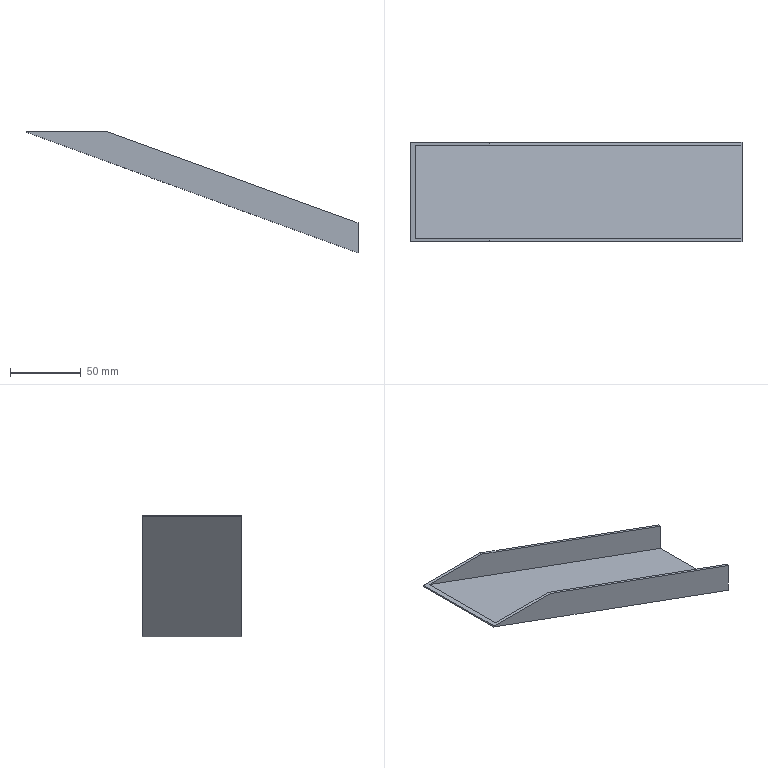Part | NX | features solid 2 | 1 solid | 11 faces | box 233.969 x 70 x 85.956 mm | volume 50310 mm3 | plane 11
STEP:
#1=CARTESIAN_POINT('',(406.321,-180.,-155.));
#2=VERTEX_POINT('',#1);
#3=CARTESIAN_POINT('',(406.031,-180.,-155.798));
#4=VERTEX_POINT('',#3);
#5=CARTESIAN_POINT('',(406.715,-180.,-153.919));
#6=DIRECTION('',(-0.342,0.,-0.9397));
#7=VECTOR('',#6,1000.);
#8=LINE('',#5,#7);
#9=EDGE_CURVE('',#2,#4,#8,.T.);
#10=ORIENTED_EDGE('',*,*,#9,.T.);
#11=CARTESIAN_POINT('',(640.,-180.,-240.956));
#12=VERTEX_POINT('',#11);
#13=CARTESIAN_POINT('',(1313.3,-180.,-486.017));
#14=DIRECTION('',(-0.9397,0.,0.342));
#15=VECTOR('',#14,1000.);
#16=LINE('',#13,#15);
#17=EDGE_CURVE('',#12,#4,#16,.T.);
#18=ORIENTED_EDGE('',*,*,#17,.F.);
#19=CARTESIAN_POINT('',(640.,-180.,-219.672));
#20=VERTEX_POINT('',#19);
#21=CARTESIAN_POINT('',(640.,-180.,-226.397));
#22=DIRECTION('',(0.,0.,1.));
#23=VECTOR('',#22,1000.);
#24=LINE('',#21,#23);
#25=EDGE_CURVE('',#12,#20,#24,.T.);
#26=ORIENTED_EDGE('',*,*,#25,.T.);
#27=CARTESIAN_POINT('',(462.314,-180.,-155.));
#28=VERTEX_POINT('',#27);
#29=CARTESIAN_POINT('',(2083.44,-180.,-745.042));
#30=DIRECTION('',(-0.9397,0.,0.342));
#31=VECTOR('',#30,1000.);
#32=LINE('',#29,#31);
#33=EDGE_CURVE('',#20,#28,#32,.T.);
#34=ORIENTED_EDGE('',*,*,#33,.T.);
#35=CARTESIAN_POINT('',(2077.284,-180.,-155.));
#36=DIRECTION('',(-1.,0.,0.));
#37=VECTOR('',#36,1000.);
#38=LINE('',#35,#37);
#39=EDGE_CURVE('',#2,#28,#38,.F.);
#40=ORIENTED_EDGE('',*,*,#39,.F.);
#41=EDGE_LOOP('',(#10,#18,#26,#34,#40));
#42=FACE_BOUND('',#41,.T.);
#43=CARTESIAN_POINT('',(2077.284,-180.,-761.956));
#44=DIRECTION('',(0.,1.,0.));
#45=DIRECTION('',(0.,0.,1.));
#46=AXIS2_PLACEMENT_3D('',#43,#44,#45);
#47=PLANE('',#46);
#48=ADVANCED_FACE('',(#42),#47,.F.);
#49=CARTESIAN_POINT('',(406.321,-110.,-155.));
#50=VERTEX_POINT('',#49);
#51=CARTESIAN_POINT('',(462.314,-110.,-155.));
#52=VERTEX_POINT('',#51);
#53=CARTESIAN_POINT('',(2077.284,-110.,-155.));
#54=DIRECTION('',(-1.,0.,0.));
#55=VECTOR('',#54,1000.);
#56=LINE('',#53,#55);
#57=EDGE_CURVE('',#50,#52,#56,.F.);
#58=ORIENTED_EDGE('',*,*,#57,.T.);
#59=CARTESIAN_POINT('',(640.,-110.,-219.672));
#60=VERTEX_POINT('',#59);
#61=CARTESIAN_POINT('',(606.84,-110.,-207.603));
#62=DIRECTION('',(-0.9397,0.,0.342));
#63=VECTOR('',#62,1000.);
#64=LINE('',#61,#63);
#65=EDGE_CURVE('',#60,#52,#64,.T.);
#66=ORIENTED_EDGE('',*,*,#65,.F.);
#67=CARTESIAN_POINT('',(640.,-110.,-240.956));
#68=VERTEX_POINT('',#67);
#69=CARTESIAN_POINT('',(640.,-110.,-226.397));
#70=DIRECTION('',(0.,0.,1.));
#71=VECTOR('',#70,1000.);
#72=LINE('',#69,#71);
#73=EDGE_CURVE('',#68,#60,#72,.T.);
#74=ORIENTED_EDGE('',*,*,#73,.F.);
#75=CARTESIAN_POINT('',(406.031,-110.,-155.798));
#76=VERTEX_POINT('',#75);
#77=CARTESIAN_POINT('',(1313.3,-110.,-486.017));
#78=DIRECTION('',(-0.9397,0.,0.342));
#79=VECTOR('',#78,1000.);
#80=LINE('',#77,#79);
#81=EDGE_CURVE('',#68,#76,#80,.T.);
#82=ORIENTED_EDGE('',*,*,#81,.T.);
#83=CARTESIAN_POINT('',(406.715,-110.,-153.919));
#84=DIRECTION('',(-0.342,0.,-0.9397));
#85=VECTOR('',#84,1000.);
#86=LINE('',#83,#85);
#87=EDGE_CURVE('',#50,#76,#86,.T.);
#88=ORIENTED_EDGE('',*,*,#87,.F.);
#89=EDGE_LOOP('',(#58,#66,#74,#82,#88));
#90=FACE_BOUND('',#89,.T.);
#91=CARTESIAN_POINT('',(2077.284,-110.,-761.956));
#92=DIRECTION('',(0.,1.,0.));
#93=DIRECTION('',(0.,0.,1.));
#94=AXIS2_PLACEMENT_3D('',#91,#92,#93);
#95=PLANE('',#94);
#96=ADVANCED_FACE('',(#90),#95,.T.);
#97=ORIENTED_EDGE('',*,*,#87,.T.);
#98=CARTESIAN_POINT('',(406.031,-706.946,-155.798));
#99=DIRECTION('',(0.,1.,0.));
#100=VECTOR('',#99,1000.);
#101=LINE('',#98,#100);
#102=EDGE_CURVE('',#4,#76,#101,.T.);
#103=ORIENTED_EDGE('',*,*,#102,.F.);
#104=ORIENTED_EDGE('',*,*,#9,.F.);
#105=CARTESIAN_POINT('',(406.321,-2357.783,-155.));
#106=DIRECTION('',(0.,1.,0.));
#107=VECTOR('',#106,1000.);
#108=LINE('',#105,#107);
#109=EDGE_CURVE('',#50,#2,#108,.F.);
#110=ORIENTED_EDGE('',*,*,#109,.F.);
#111=EDGE_LOOP('',(#97,#103,#104,#110));
#112=FACE_BOUND('',#111,.T.);
#113=CARTESIAN_POINT('',(406.715,-2357.783,-153.919));
#114=DIRECTION('',(0.9397,0.,-0.342));
#115=DIRECTION('',(0.342,0.,0.9397));
#116=AXIS2_PLACEMENT_3D('',#113,#114,#115);
#117=PLANE('',#116);
#118=ADVANCED_FACE('',(#112),#117,.F.);
#119=CARTESIAN_POINT('',(640.,-112.,-238.827));
#120=VERTEX_POINT('',#119);
#121=CARTESIAN_POINT('',(409.686,-112.,-155.));
#122=VERTEX_POINT('',#121);
#123=CARTESIAN_POINT('',(1313.984,-112.,-484.138));
#124=DIRECTION('',(-0.9397,0.,0.342));
#125=VECTOR('',#124,1000.);
#126=LINE('',#123,#125);
#127=EDGE_CURVE('',#120,#122,#126,.T.);
#128=ORIENTED_EDGE('',*,*,#127,.F.);
#129=CARTESIAN_POINT('',(640.,-112.,-219.672));
#130=VERTEX_POINT('',#129);
#131=CARTESIAN_POINT('',(640.,-112.,-226.397));
#132=DIRECTION('',(0.,0.,-1.));
#133=VECTOR('',#132,1000.);
#134=LINE('',#131,#133);
#135=EDGE_CURVE('',#130,#120,#134,.T.);
#136=ORIENTED_EDGE('',*,*,#135,.F.);
#137=CARTESIAN_POINT('',(462.314,-112.,-155.));
#138=VERTEX_POINT('',#137);
#139=CARTESIAN_POINT('',(606.84,-112.,-207.603));
#140=DIRECTION('',(-0.9397,0.,0.342));
#141=VECTOR('',#140,1000.);
#142=LINE('',#139,#141);
#143=EDGE_CURVE('',#130,#138,#142,.T.);
#144=ORIENTED_EDGE('',*,*,#143,.T.);
#145=CARTESIAN_POINT('',(600.,-112.,-155.));
#146=DIRECTION('',(-1.,0.,0.));
#147=VECTOR('',#146,1000.);
#148=LINE('',#145,#147);
#149=EDGE_CURVE('',#122,#138,#148,.F.);
#150=ORIENTED_EDGE('',*,*,#149,.F.);
#151=EDGE_LOOP('',(#128,#136,#144,#150));
#152=FACE_BOUND('',#151,.T.);
#153=CARTESIAN_POINT('',(600.,-112.,-226.397));
#154=DIRECTION('',(0.,1.,0.));
#155=DIRECTION('',(-0.9397,0.,0.342));
#156=AXIS2_PLACEMENT_3D('',#153,#154,#155);
#157=PLANE('',#156);
#158=ADVANCED_FACE('',(#152),#157,.F.);
#159=ORIENTED_EDGE('',*,*,#143,.F.);
#160=CARTESIAN_POINT('',(640.,-90.,-219.672));
#161=DIRECTION('',(0.,-1.,0.));
#162=VECTOR('',#161,1000.);
#163=LINE('',#160,#162);
#164=EDGE_CURVE('',#60,#130,#163,.T.);
#165=ORIENTED_EDGE('',*,*,#164,.F.);
#166=ORIENTED_EDGE('',*,*,#65,.T.);
#167=CARTESIAN_POINT('',(462.314,-90.,-155.));
#168=DIRECTION('',(0.,-1.,0.));
#169=VECTOR('',#168,1000.);
#170=LINE('',#167,#169);
#171=EDGE_CURVE('',#138,#52,#170,.F.);
#172=ORIENTED_EDGE('',*,*,#171,.F.);
#173=EDGE_LOOP('',(#159,#165,#166,#172));
#174=FACE_BOUND('',#173,.T.);
#175=CARTESIAN_POINT('',(606.84,-90.,-207.603));
#176=DIRECTION('',(-0.342,0.,-0.9397));
#177=DIRECTION('',(0.9397,0.,-0.342));
#178=AXIS2_PLACEMENT_3D('',#175,#176,#177);
#179=PLANE('',#178);
#180=ADVANCED_FACE('',(#174),#179,.F.);
#181=CARTESIAN_POINT('',(640.,-178.,-219.672));
#182=VERTEX_POINT('',#181);
#183=CARTESIAN_POINT('',(462.314,-178.,-155.));
#184=VERTEX_POINT('',#183);
#185=CARTESIAN_POINT('',(606.84,-178.,-207.603));
#186=DIRECTION('',(-0.9397,0.,0.342));
#187=VECTOR('',#186,1000.);
#188=LINE('',#185,#187);
#189=EDGE_CURVE('',#182,#184,#188,.T.);
#190=ORIENTED_EDGE('',*,*,#189,.F.);
#191=CARTESIAN_POINT('',(640.,-178.,-238.827));
#192=VERTEX_POINT('',#191);
#193=CARTESIAN_POINT('',(640.,-178.,-226.397));
#194=DIRECTION('',(0.,0.,1.));
#195=VECTOR('',#194,1000.);
#196=LINE('',#193,#195);
#197=EDGE_CURVE('',#192,#182,#196,.T.);
#198=ORIENTED_EDGE('',*,*,#197,.F.);
#199=CARTESIAN_POINT('',(409.686,-178.,-155.));
#200=VERTEX_POINT('',#199);
#201=CARTESIAN_POINT('',(1313.984,-178.,-484.138));
#202=DIRECTION('',(0.9397,0.,-0.342));
#203=VECTOR('',#202,1000.);
#204=LINE('',#201,#203);
#205=EDGE_CURVE('',#200,#192,#204,.T.);
#206=ORIENTED_EDGE('',*,*,#205,.F.);
#207=CARTESIAN_POINT('',(600.,-178.,-155.));
#208=DIRECTION('',(1.,0.,0.));
#209=VECTOR('',#208,1000.);
#210=LINE('',#207,#209);
#211=EDGE_CURVE('',#184,#200,#210,.F.);
#212=ORIENTED_EDGE('',*,*,#211,.F.);
#213=EDGE_LOOP('',(#190,#198,#206,#212));
#214=FACE_BOUND('',#213,.T.);
#215=CARTESIAN_POINT('',(600.,-178.,-226.397));
#216=DIRECTION('',(0.,-1.,0.));
#217=DIRECTION('',(-0.9397,0.,0.342));
#218=AXIS2_PLACEMENT_3D('',#215,#216,#217);
#219=PLANE('',#218);
#220=ADVANCED_FACE('',(#214),#219,.F.);
#221=CARTESIAN_POINT('',(462.314,-190.,-155.));
#222=DIRECTION('',(0.,1.,0.));
#223=VECTOR('',#222,1000.);
#224=LINE('',#221,#223);
#225=EDGE_CURVE('',#184,#28,#224,.F.);
#226=ORIENTED_EDGE('',*,*,#225,.T.);
#227=ORIENTED_EDGE('',*,*,#33,.F.);
#228=CARTESIAN_POINT('',(640.,-190.,-219.672));
#229=DIRECTION('',(0.,1.,0.));
#230=VECTOR('',#229,1000.);
#231=LINE('',#228,#230);
#232=EDGE_CURVE('',#20,#182,#231,.T.);
#233=ORIENTED_EDGE('',*,*,#232,.T.);
#234=ORIENTED_EDGE('',*,*,#189,.T.);
#235=EDGE_LOOP('',(#226,#227,#233,#234));
#236=FACE_BOUND('',#235,.T.);
#237=CARTESIAN_POINT('',(606.84,-190.,-207.603));
#238=DIRECTION('',(0.342,0.,0.9397));
#239=DIRECTION('',(-0.9397,0.,0.342));
#240=AXIS2_PLACEMENT_3D('',#237,#238,#239);
#241=PLANE('',#240);
#242=ADVANCED_FACE('',(#236),#241,.T.);
#243=ORIENTED_EDGE('',*,*,#205,.T.);
#244=CARTESIAN_POINT('',(640.,-706.946,-238.827));
#245=DIRECTION('',(0.,-1.,0.));
#246=VECTOR('',#245,1000.);
#247=LINE('',#244,#246);
#248=EDGE_CURVE('',#120,#192,#247,.T.);
#249=ORIENTED_EDGE('',*,*,#248,.F.);
#250=ORIENTED_EDGE('',*,*,#127,.T.);
#251=CARTESIAN_POINT('',(409.686,-706.946,-155.));
#252=DIRECTION('',(0.,-1.,0.));
#253=VECTOR('',#252,1000.);
#254=LINE('',#251,#253);
#255=EDGE_CURVE('',#200,#122,#254,.F.);
#256=ORIENTED_EDGE('',*,*,#255,.F.);
#257=EDGE_LOOP('',(#243,#249,#250,#256));
#258=FACE_BOUND('',#257,.T.);
#259=CARTESIAN_POINT('',(1313.984,-706.946,-484.138));
#260=DIRECTION('',(-0.342,0.,-0.9397));
#261=DIRECTION('',(0.9397,0.,-0.342));
#262=AXIS2_PLACEMENT_3D('',#259,#260,#261);
#263=PLANE('',#262);
#264=ADVANCED_FACE('',(#258),#263,.F.);
#265=CARTESIAN_POINT('',(640.,-190.,-240.956));
#266=DIRECTION('',(0.,1.,0.));
#267=VECTOR('',#266,1000.);
#268=LINE('',#265,#267);
#269=EDGE_CURVE('',#12,#68,#268,.T.);
#270=ORIENTED_EDGE('',*,*,#269,.F.);
#271=ORIENTED_EDGE('',*,*,#17,.T.);
#272=ORIENTED_EDGE('',*,*,#102,.T.);
#273=ORIENTED_EDGE('',*,*,#81,.F.);
#274=EDGE_LOOP('',(#270,#271,#272,#273));
#275=FACE_BOUND('',#274,.T.);
#276=CARTESIAN_POINT('',(1313.3,-706.946,-486.017));
#277=DIRECTION('',(-0.342,0.,-0.9397));
#278=DIRECTION('',(0.9397,0.,-0.342));
#279=AXIS2_PLACEMENT_3D('',#276,#277,#278);
#280=PLANE('',#279);
#281=ADVANCED_FACE('',(#275),#280,.T.);
#282=ORIENTED_EDGE('',*,*,#73,.T.);
#283=ORIENTED_EDGE('',*,*,#164,.T.);
#284=ORIENTED_EDGE('',*,*,#135,.T.);
#285=ORIENTED_EDGE('',*,*,#248,.T.);
#286=ORIENTED_EDGE('',*,*,#197,.T.);
#287=ORIENTED_EDGE('',*,*,#232,.F.);
#288=ORIENTED_EDGE('',*,*,#25,.F.);
#289=ORIENTED_EDGE('',*,*,#269,.T.);
#290=EDGE_LOOP('',(#282,#283,#284,#285,#286,#287,#288,#289));
#291=FACE_BOUND('',#290,.T.);
#292=CARTESIAN_POINT('',(640.,-190.,-226.397));
#293=DIRECTION('',(-1.,0.,0.));
#294=DIRECTION('',(0.,0.,-1.));
#295=AXIS2_PLACEMENT_3D('',#292,#293,#294);
#296=PLANE('',#295);
#297=ADVANCED_FACE('',(#291),#296,.F.);
#298=ORIENTED_EDGE('',*,*,#109,.T.);
#299=ORIENTED_EDGE('',*,*,#39,.T.);
#300=ORIENTED_EDGE('',*,*,#225,.F.);
#301=ORIENTED_EDGE('',*,*,#211,.T.);
#302=ORIENTED_EDGE('',*,*,#255,.T.);
#303=ORIENTED_EDGE('',*,*,#149,.T.);
#304=ORIENTED_EDGE('',*,*,#171,.T.);
#305=ORIENTED_EDGE('',*,*,#57,.F.);
#306=EDGE_LOOP('',(#298,#299,#300,#301,#302,#303,#304,#305));
#307=FACE_BOUND('',#306,.T.);
#308=CARTESIAN_POINT('',(0.,-2277.783,-155.));
#309=DIRECTION('',(0.,0.,1.));
#310=DIRECTION('',(0.,1.,0.));
#311=AXIS2_PLACEMENT_3D('',#308,#309,#310);
#312=PLANE('',#311);
#313=ADVANCED_FACE('',(#307),#312,.T.);
#314=CLOSED_SHELL('',(#48,#96,#118,#158,#180,#220,#242,#264,#281,#297,#313));
#315=MANIFOLD_SOLID_BREP('',#314);
#316=(LENGTH_UNIT()NAMED_UNIT(*)SI_UNIT(.MILLI.,.METRE.));
#317=UNCERTAINTY_MEASURE_WITH_UNIT(LENGTH_MEASURE(0.00001),#316,'','');
#318=(NAMED_UNIT(*)PLANE_ANGLE_UNIT()SI_UNIT($,.RADIAN.));
#319=(NAMED_UNIT(*)SI_UNIT($,.STERADIAN.)SOLID_ANGLE_UNIT());
#320=(GEOMETRIC_REPRESENTATION_CONTEXT(3)GLOBAL_UNCERTAINTY_ASSIGNED_CONTEXT((#317))GLOBAL_UNIT_ASSIGNED_CONTEXT((#316,#318,#319))REPRESENTATION_CONTEXT('',''));
#321=ADVANCED_BREP_SHAPE_REPRESENTATION('',(#315),#320);